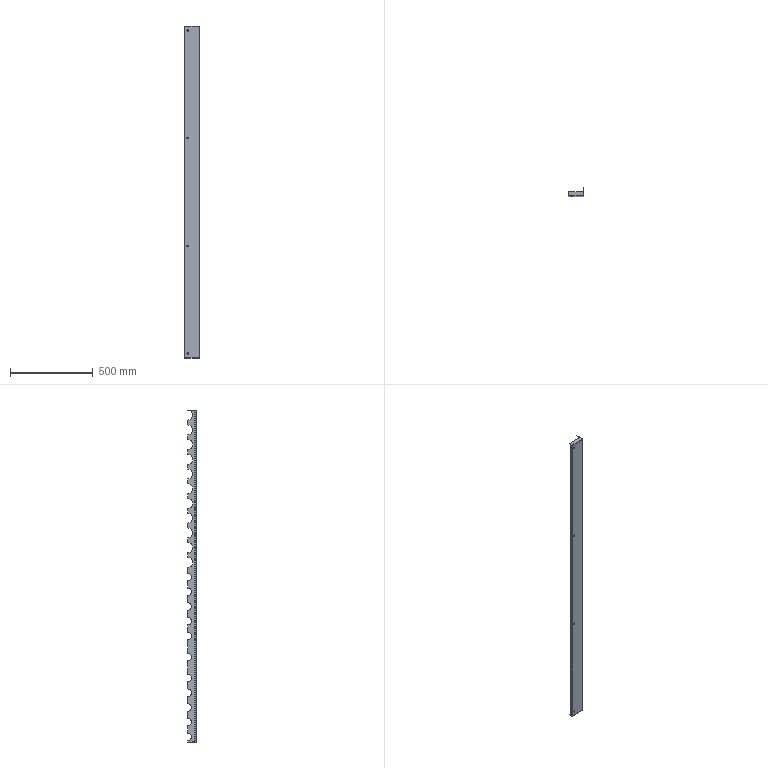Part | SolidWorks | features BaseBody 1 | 1 solid | 94 faces | box 95 x 51.5 x 2005 mm | volume 427193 mm3 | plane 56 | cylinder 38 | commonest cylinder face diameters 45 x11 60 x11 9 x8 1.473 x4 4.473 x4